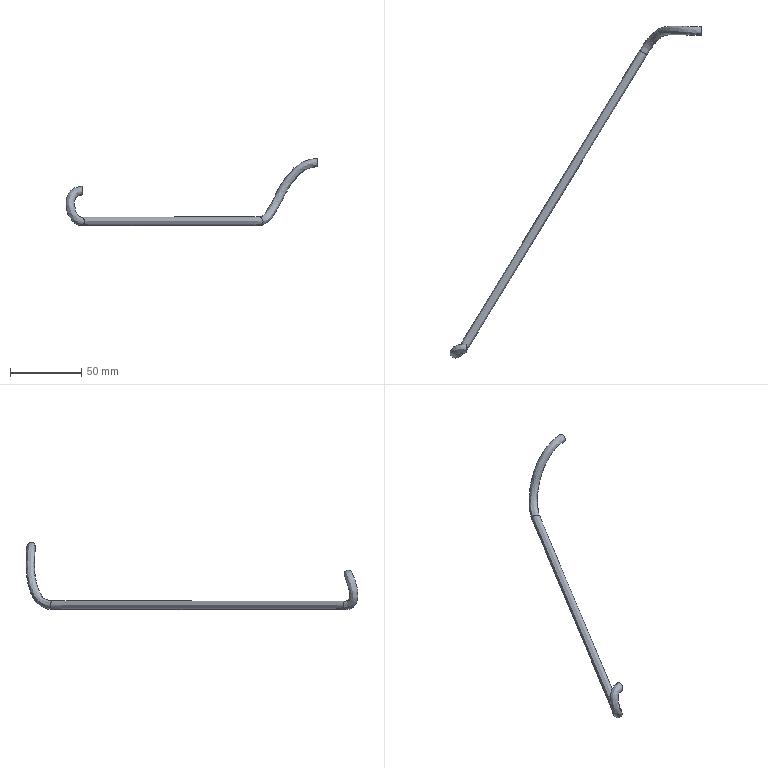Part | NX | features solid 2 | 1 solid | 8 faces | box 176.431 x 232.411 x 47.002 mm | volume 5345 mm3 | spline 6 | plane 2